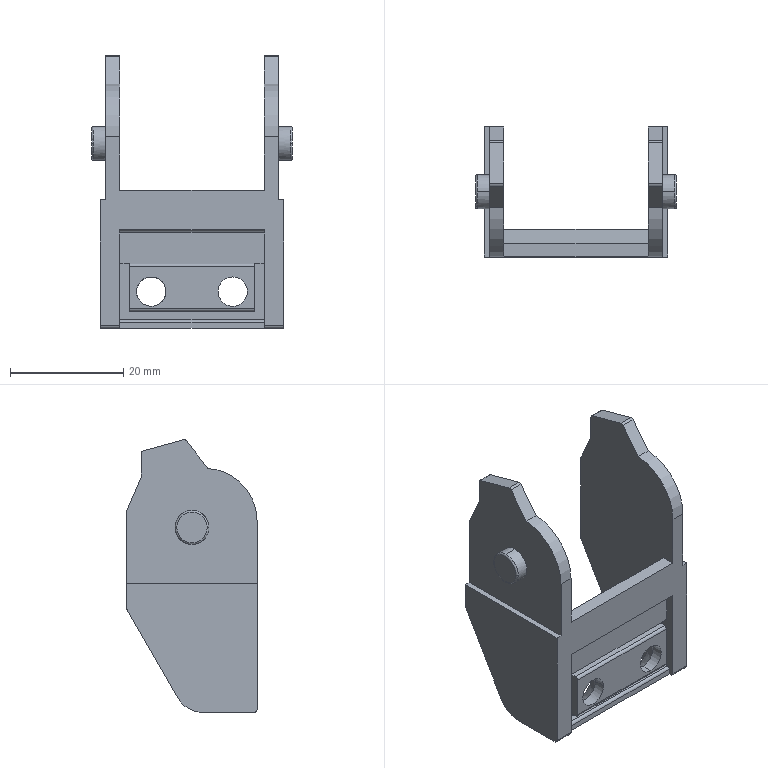Part | SolidWorks | features BaseBody 1 | 1 solid | 76 faces | box 35.5 x 23 x 48.229 mm | volume 7278 mm3 | plane 42 | cylinder 26 | cone 4 | torus 4 | commonest cylinder face diameters 1 x14 5.2 x4 6 x4 10 x2 18.6 x2